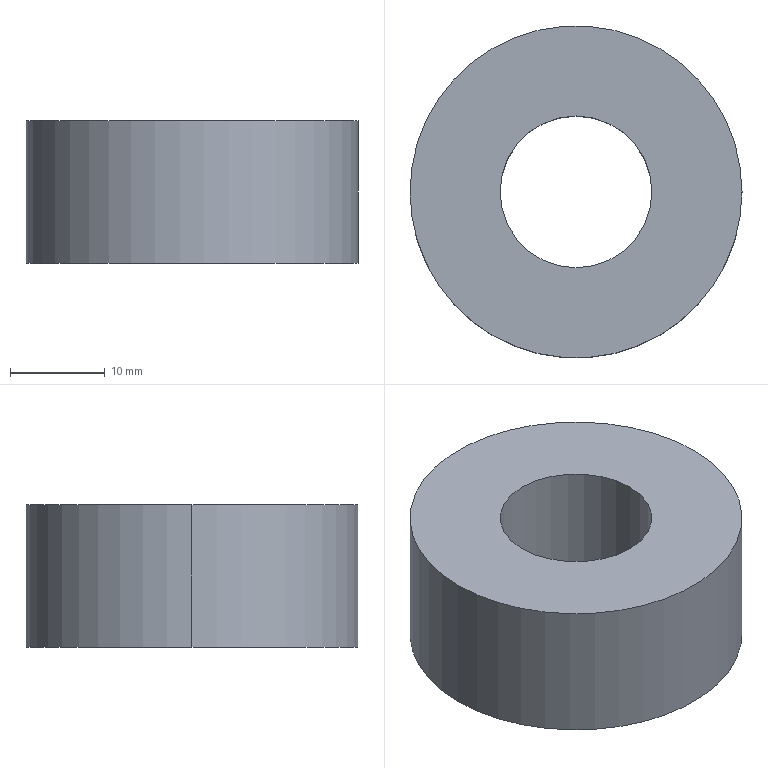Part | SolidWorks | features Extrusion 1 | 1 solid | 6 faces | box 35 x 35 x 15 mm | volume 11416 mm3 | cylinder 4 | plane 2 | commonest cylinder face diameters 16 x2 35 x2
STEP:
#1=CARTESIAN_POINT('',(-8.,0.,7.5));
#2=VERTEX_POINT('',#1);
#3=CARTESIAN_POINT('',(8.,0.,7.5));
#4=VERTEX_POINT('',#3);
#5=CARTESIAN_POINT('',(0.,0.,7.5));
#6=DIRECTION('',(0.,0.,1.));
#7=DIRECTION('',(1.,0.,0.));
#8=AXIS2_PLACEMENT_3D('',#5,#6,#7);
#9=CIRCLE('',#8,8.);
#10=EDGE_CURVE('',#2,#4,#9,.T.);
#11=ORIENTED_EDGE('',*,*,#10,.T.);
#12=CARTESIAN_POINT('',(8.,0.,-7.5));
#13=VERTEX_POINT('',#12);
#14=CARTESIAN_POINT('',(8.,0.,7.5));
#15=DIRECTION('',(0.,0.,-1.));
#16=VECTOR('',#15,1000.);
#17=LINE('',#14,#16);
#18=EDGE_CURVE('',#4,#13,#17,.T.);
#19=ORIENTED_EDGE('',*,*,#18,.T.);
#20=CARTESIAN_POINT('',(-8.,0.,-7.5));
#21=VERTEX_POINT('',#20);
#22=CARTESIAN_POINT('',(0.,0.,-7.5));
#23=DIRECTION('',(0.,0.,1.));
#24=DIRECTION('',(1.,0.,0.));
#25=AXIS2_PLACEMENT_3D('',#22,#23,#24);
#26=CIRCLE('',#25,8.);
#27=EDGE_CURVE('',#21,#13,#26,.T.);
#28=ORIENTED_EDGE('',*,*,#27,.F.);
#29=CARTESIAN_POINT('',(-8.,0.,7.5));
#30=DIRECTION('',(0.,0.,-1.));
#31=VECTOR('',#30,1000.);
#32=LINE('',#29,#31);
#33=EDGE_CURVE('',#2,#21,#32,.T.);
#34=ORIENTED_EDGE('',*,*,#33,.F.);
#35=EDGE_LOOP('',(#11,#19,#28,#34));
#36=FACE_OUTER_BOUND('',#35,.T.);
#37=CARTESIAN_POINT('',(0.,0.,7.5));
#38=DIRECTION('',(0.,0.,-1.));
#39=DIRECTION('',(-1.,0.,0.));
#40=AXIS2_PLACEMENT_3D('',#37,#38,#39);
#41=CYLINDRICAL_SURFACE('',#40,8.);
#42=ADVANCED_FACE('',(#36),#41,.F.);
#43=CARTESIAN_POINT('',(17.5,0.,7.5));
#44=VERTEX_POINT('',#43);
#45=CARTESIAN_POINT('',(-17.5,0.,7.5));
#46=VERTEX_POINT('',#45);
#47=CARTESIAN_POINT('',(0.,0.,7.5));
#48=DIRECTION('',(0.,0.,1.));
#49=DIRECTION('',(1.,0.,0.));
#50=AXIS2_PLACEMENT_3D('',#47,#48,#49);
#51=CIRCLE('',#50,17.5);
#52=EDGE_CURVE('',#44,#46,#51,.T.);
#53=ORIENTED_EDGE('',*,*,#52,.F.);
#54=CARTESIAN_POINT('',(17.5,0.,-7.5));
#55=VERTEX_POINT('',#54);
#56=CARTESIAN_POINT('',(17.5,0.,7.5));
#57=DIRECTION('',(0.,0.,-1.));
#58=VECTOR('',#57,1000.);
#59=LINE('',#56,#58);
#60=EDGE_CURVE('',#44,#55,#59,.T.);
#61=ORIENTED_EDGE('',*,*,#60,.T.);
#62=CARTESIAN_POINT('',(-17.5,0.,-7.5));
#63=VERTEX_POINT('',#62);
#64=CARTESIAN_POINT('',(0.,0.,-7.5));
#65=DIRECTION('',(0.,0.,1.));
#66=DIRECTION('',(1.,0.,0.));
#67=AXIS2_PLACEMENT_3D('',#64,#65,#66);
#68=CIRCLE('',#67,17.5);
#69=EDGE_CURVE('',#55,#63,#68,.T.);
#70=ORIENTED_EDGE('',*,*,#69,.T.);
#71=CARTESIAN_POINT('',(-17.5,0.,7.5));
#72=DIRECTION('',(0.,0.,-1.));
#73=VECTOR('',#72,1000.);
#74=LINE('',#71,#73);
#75=EDGE_CURVE('',#46,#63,#74,.T.);
#76=ORIENTED_EDGE('',*,*,#75,.F.);
#77=EDGE_LOOP('',(#53,#61,#70,#76));
#78=FACE_OUTER_BOUND('',#77,.T.);
#79=CARTESIAN_POINT('',(0.,0.,7.5));
#80=DIRECTION('',(0.,0.,-1.));
#81=DIRECTION('',(-1.,0.,0.));
#82=AXIS2_PLACEMENT_3D('',#79,#80,#81);
#83=CYLINDRICAL_SURFACE('',#82,17.5);
#84=ADVANCED_FACE('',(#78),#83,.T.);
#85=CARTESIAN_POINT('',(0.,0.,7.5));
#86=DIRECTION('',(0.,0.,1.));
#87=DIRECTION('',(1.,0.,0.));
#88=AXIS2_PLACEMENT_3D('',#85,#86,#87);
#89=CIRCLE('',#88,17.5);
#90=EDGE_CURVE('',#46,#44,#89,.T.);
#91=ORIENTED_EDGE('',*,*,#90,.T.);
#92=ORIENTED_EDGE('',*,*,#52,.T.);
#93=EDGE_LOOP('',(#91,#92));
#94=FACE_OUTER_BOUND('',#93,.T.);
#95=ORIENTED_EDGE('',*,*,#10,.F.);
#96=CARTESIAN_POINT('',(0.,0.,7.5));
#97=DIRECTION('',(0.,0.,1.));
#98=DIRECTION('',(1.,0.,0.));
#99=AXIS2_PLACEMENT_3D('',#96,#97,#98);
#100=CIRCLE('',#99,8.);
#101=EDGE_CURVE('',#4,#2,#100,.T.);
#102=ORIENTED_EDGE('',*,*,#101,.F.);
#103=EDGE_LOOP('',(#95,#102));
#104=FACE_BOUND('',#103,.T.);
#105=CARTESIAN_POINT('',(0.,0.,7.5));
#106=DIRECTION('',(0.,0.,1.));
#107=DIRECTION('',(1.,0.,0.));
#108=AXIS2_PLACEMENT_3D('',#105,#106,#107);
#109=PLANE('',#108);
#110=ADVANCED_FACE('',(#94,#104),#109,.T.);
#111=CARTESIAN_POINT('',(0.,0.,-7.5));
#112=DIRECTION('',(0.,0.,1.));
#113=DIRECTION('',(1.,0.,0.));
#114=AXIS2_PLACEMENT_3D('',#111,#112,#113);
#115=CIRCLE('',#114,17.5);
#116=EDGE_CURVE('',#63,#55,#115,.T.);
#117=ORIENTED_EDGE('',*,*,#116,.F.);
#118=ORIENTED_EDGE('',*,*,#69,.F.);
#119=EDGE_LOOP('',(#117,#118));
#120=FACE_OUTER_BOUND('',#119,.T.);
#121=ORIENTED_EDGE('',*,*,#27,.T.);
#122=CARTESIAN_POINT('',(0.,0.,-7.5));
#123=DIRECTION('',(0.,0.,1.));
#124=DIRECTION('',(1.,0.,0.));
#125=AXIS2_PLACEMENT_3D('',#122,#123,#124);
#126=CIRCLE('',#125,8.);
#127=EDGE_CURVE('',#13,#21,#126,.T.);
#128=ORIENTED_EDGE('',*,*,#127,.T.);
#129=EDGE_LOOP('',(#121,#128));
#130=FACE_BOUND('',#129,.T.);
#131=CARTESIAN_POINT('',(0.,0.,-7.5));
#132=DIRECTION('',(0.,0.,1.));
#133=DIRECTION('',(1.,0.,0.));
#134=AXIS2_PLACEMENT_3D('',#131,#132,#133);
#135=PLANE('',#134);
#136=ADVANCED_FACE('',(#120,#130),#135,.F.);
#137=ORIENTED_EDGE('',*,*,#60,.F.);
#138=ORIENTED_EDGE('',*,*,#90,.F.);
#139=ORIENTED_EDGE('',*,*,#75,.T.);
#140=ORIENTED_EDGE('',*,*,#116,.T.);
#141=EDGE_LOOP('',(#137,#138,#139,#140));
#142=FACE_OUTER_BOUND('',#141,.T.);
#143=CARTESIAN_POINT('',(0.,0.,7.5));
#144=DIRECTION('',(0.,0.,-1.));
#145=DIRECTION('',(-1.,0.,0.));
#146=AXIS2_PLACEMENT_3D('',#143,#144,#145);
#147=CYLINDRICAL_SURFACE('',#146,17.5);
#148=ADVANCED_FACE('',(#142),#147,.T.);
#149=ORIENTED_EDGE('',*,*,#18,.F.);
#150=ORIENTED_EDGE('',*,*,#101,.T.);
#151=ORIENTED_EDGE('',*,*,#33,.T.);
#152=ORIENTED_EDGE('',*,*,#127,.F.);
#153=EDGE_LOOP('',(#149,#150,#151,#152));
#154=FACE_OUTER_BOUND('',#153,.T.);
#155=CARTESIAN_POINT('',(0.,0.,7.5));
#156=DIRECTION('',(0.,0.,-1.));
#157=DIRECTION('',(-1.,0.,0.));
#158=AXIS2_PLACEMENT_3D('',#155,#156,#157);
#159=CYLINDRICAL_SURFACE('',#158,8.);
#160=ADVANCED_FACE('',(#154),#159,.F.);
#161=CLOSED_SHELL('',(#42,#84,#110,#136,#148,#160));
#162=MANIFOLD_SOLID_BREP('',#161);
#163=CARTESIAN_POINT('',(0.,0.,0.));
#164=DIRECTION('',(0.,0.,1.));
#165=DIRECTION('',(1.,0.,0.));
#166=AXIS2_PLACEMENT_3D('',#163,#164,#165);
#167=(LENGTH_UNIT()NAMED_UNIT(*)SI_UNIT(.MILLI.,.METRE.));
#168=UNCERTAINTY_MEASURE_WITH_UNIT(LENGTH_MEASURE(0.00001),#167,'','');
#169=(NAMED_UNIT(*)PLANE_ANGLE_UNIT()SI_UNIT($,.RADIAN.));
#170=(NAMED_UNIT(*)SI_UNIT($,.STERADIAN.)SOLID_ANGLE_UNIT());
#171=(GEOMETRIC_REPRESENTATION_CONTEXT(3)GLOBAL_UNCERTAINTY_ASSIGNED_CONTEXT((#168))GLOBAL_UNIT_ASSIGNED_CONTEXT((#167,#169,#170))REPRESENTATION_CONTEXT('',''));
#172=ADVANCED_BREP_SHAPE_REPRESENTATION('',(#162,#166),#171);